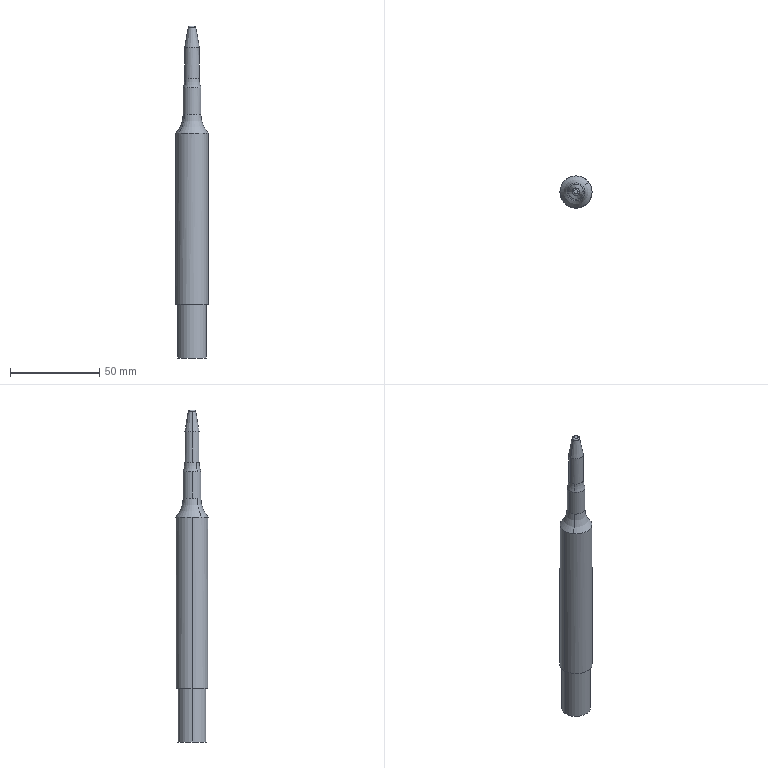Part | 1 solid | 19 faces | box 18 x 18 x 186 mm | volume 34533 mm3 | cylinder 8 | torus 6 | plane 3 | cone 2 | commonest cylinder face diameters 8.2 x2 9.9 x2 16 x2 18 x2
STEP:
#1=CARTESIAN_POINT('',(0.,0.,0.));
#2=DIRECTION('',(0.,0.,1.));
#3=DIRECTION('',(1.,0.,0.));
#4=AXIS2_PLACEMENT_3D('',#1,#2,#3);
#5=CARTESIAN_POINT('',(-232.,180.5,-322.55));
#6=VERTEX_POINT('',#5);
#7=CARTESIAN_POINT('',(-248.,180.5,-322.55));
#8=VERTEX_POINT('',#7);
#9=CARTESIAN_POINT('',(-240.,180.5,-322.55));
#10=DIRECTION('',(0.,0.,1.));
#11=DIRECTION('',(1.,0.,0.));
#12=AXIS2_PLACEMENT_3D('',#9,#10,#11);
#13=CIRCLE('',#12,8.);
#14=CARTESIAN_POINT('',(-226.,4.5,-322.55));
#15=DIRECTION('',(0.,0.,1.));
#16=DIRECTION('',(0.,1.,0.));
#17=AXIS2_PLACEMENT_3D('',#14,#15,#16);
#18=PLANE('',#17);
#19=CARTESIAN_POINT('',(176.,14.));
#20=DIRECTION('',(0.,-1.));
#21=AXIS2_PLACEMENT_2D('',#19,#20);
#22=CIRCLE('',#21,8.);
#23=(GEOMETRIC_REPRESENTATION_CONTEXT(2)PARAMETRIC_REPRESENTATION_CONTEXT()REPRESENTATION_CONTEXT('',''));
#24=DEFINITIONAL_REPRESENTATION('',(#22),#23);
#25=PCURVE('',#18,#24);
#26=CARTESIAN_POINT('',(-240.,180.5,-342.55));
#27=DIRECTION('',(0.,0.,1.));
#28=DIRECTION('',(0.,-1.,0.));
#29=AXIS2_PLACEMENT_3D('',#26,#27,#28);
#30=CYLINDRICAL_SURFACE('',#29,8.);
#31=CARTESIAN_POINT('',(1.571,20.));
#32=DIRECTION('',(1.,0.));
#33=VECTOR('',#32,1.);
#34=LINE('',#31,#33);
#35=(GEOMETRIC_REPRESENTATION_CONTEXT(2)PARAMETRIC_REPRESENTATION_CONTEXT()REPRESENTATION_CONTEXT('',''));
#36=DEFINITIONAL_REPRESENTATION('',(#34),#35);
#37=PCURVE('',#30,#36);
#38=SURFACE_CURVE('',#13,(#25,#37),.PCURVE_S1.);
#39=EDGE_CURVE('',#6,#8,#38,.T.);
#40=ORIENTED_EDGE('',*,*,#39,.T.);
#41=CARTESIAN_POINT('',(-240.,180.5,-322.55));
#42=DIRECTION('',(0.,0.,1.));
#43=DIRECTION('',(1.,0.,0.));
#44=AXIS2_PLACEMENT_3D('',#41,#42,#43);
#45=CIRCLE('',#44,8.);
#46=CARTESIAN_POINT('',(176.,14.));
#47=DIRECTION('',(0.,-1.));
#48=AXIS2_PLACEMENT_2D('',#46,#47);
#49=CIRCLE('',#48,8.);
#50=(GEOMETRIC_REPRESENTATION_CONTEXT(2)PARAMETRIC_REPRESENTATION_CONTEXT()REPRESENTATION_CONTEXT('',''));
#51=DEFINITIONAL_REPRESENTATION('',(#49),#50);
#52=PCURVE('',#18,#51);
#53=CARTESIAN_POINT('',(-240.,180.5,-342.55));
#54=DIRECTION('',(0.,0.,1.));
#55=DIRECTION('',(0.,1.,0.));
#56=AXIS2_PLACEMENT_3D('',#53,#54,#55);
#57=CYLINDRICAL_SURFACE('',#56,8.);
#58=CARTESIAN_POINT('',(-1.571,20.));
#59=DIRECTION('',(1.,0.));
#60=VECTOR('',#59,1.);
#61=LINE('',#58,#60);
#62=(GEOMETRIC_REPRESENTATION_CONTEXT(2)PARAMETRIC_REPRESENTATION_CONTEXT()REPRESENTATION_CONTEXT('',''));
#63=DEFINITIONAL_REPRESENTATION('',(#61),#62);
#64=PCURVE('',#57,#63);
#65=SURFACE_CURVE('',#45,(#52,#64),.PCURVE_S1.);
#66=EDGE_CURVE('',#8,#6,#65,.T.);
#67=ORIENTED_EDGE('',*,*,#66,.T.);
#68=EDGE_LOOP('',(#40,#67));
#69=FACE_BOUND('',#68,.T.);
#70=CARTESIAN_POINT('',(-231.,180.5,-322.55));
#71=VERTEX_POINT('',#70);
#72=CARTESIAN_POINT('',(-249.,180.5,-322.55));
#73=VERTEX_POINT('',#72);
#74=CARTESIAN_POINT('',(-240.,180.5,-322.55));
#75=DIRECTION('',(0.,0.,1.));
#76=DIRECTION('',(-1.,0.,0.));
#77=AXIS2_PLACEMENT_3D('',#74,#75,#76);
#78=CIRCLE('',#77,9.);
#79=CARTESIAN_POINT('',(176.,14.));
#80=DIRECTION('',(0.,1.));
#81=AXIS2_PLACEMENT_2D('',#79,#80);
#82=CIRCLE('',#81,9.);
#83=(GEOMETRIC_REPRESENTATION_CONTEXT(2)PARAMETRIC_REPRESENTATION_CONTEXT()REPRESENTATION_CONTEXT('',''));
#84=DEFINITIONAL_REPRESENTATION('',(#82),#83);
#85=PCURVE('',#18,#84);
#86=CARTESIAN_POINT('',(-240.,180.5,-306.55));
#87=DIRECTION('',(0.,0.,1.));
#88=DIRECTION('',(0.,-1.,0.));
#89=AXIS2_PLACEMENT_3D('',#86,#87,#88);
#90=CYLINDRICAL_SURFACE('',#89,9.);
#91=CARTESIAN_POINT('',(-1.571,-16.));
#92=DIRECTION('',(1.,0.));
#93=VECTOR('',#92,1.);
#94=LINE('',#91,#93);
#95=(GEOMETRIC_REPRESENTATION_CONTEXT(2)PARAMETRIC_REPRESENTATION_CONTEXT()REPRESENTATION_CONTEXT('',''));
#96=DEFINITIONAL_REPRESENTATION('',(#94),#95);
#97=PCURVE('',#90,#96);
#98=SURFACE_CURVE('',#78,(#85,#97),.PCURVE_S1.);
#99=EDGE_CURVE('',#71,#73,#98,.T.);
#100=ORIENTED_EDGE('',*,*,#99,.F.);
#101=CARTESIAN_POINT('',(-240.,180.5,-322.55));
#102=DIRECTION('',(0.,0.,1.));
#103=DIRECTION('',(-1.,0.,0.));
#104=AXIS2_PLACEMENT_3D('',#101,#102,#103);
#105=CIRCLE('',#104,9.);
#106=CARTESIAN_POINT('',(176.,14.));
#107=DIRECTION('',(0.,1.));
#108=AXIS2_PLACEMENT_2D('',#106,#107);
#109=CIRCLE('',#108,9.);
#110=(GEOMETRIC_REPRESENTATION_CONTEXT(2)PARAMETRIC_REPRESENTATION_CONTEXT()REPRESENTATION_CONTEXT('',''));
#111=DEFINITIONAL_REPRESENTATION('',(#109),#110);
#112=PCURVE('',#18,#111);
#113=CARTESIAN_POINT('',(-240.,180.5,-306.55));
#114=DIRECTION('',(0.,0.,1.));
#115=DIRECTION('',(0.,1.,0.));
#116=AXIS2_PLACEMENT_3D('',#113,#114,#115);
#117=CYLINDRICAL_SURFACE('',#116,9.);
#118=CARTESIAN_POINT('',(1.571,-16.));
#119=DIRECTION('',(1.,0.));
#120=VECTOR('',#119,1.);
#121=LINE('',#118,#120);
#122=(GEOMETRIC_REPRESENTATION_CONTEXT(2)PARAMETRIC_REPRESENTATION_CONTEXT()REPRESENTATION_CONTEXT('',''));
#123=DEFINITIONAL_REPRESENTATION('',(#121),#122);
#124=PCURVE('',#117,#123);
#125=SURFACE_CURVE('',#105,(#112,#124),.PCURVE_S1.);
#126=EDGE_CURVE('',#73,#71,#125,.T.);
#127=ORIENTED_EDGE('',*,*,#126,.F.);
#128=EDGE_LOOP('',(#100,#127));
#129=FACE_BOUND('',#128,.T.);
#130=ADVANCED_FACE('',(#69,#129),#18,.F.);
#131=CARTESIAN_POINT('',(-231.,180.5,-226.55));
#132=VERTEX_POINT('',#131);
#133=CARTESIAN_POINT('',(-231.,180.5,-322.55));
#134=DIRECTION('',(0.,0.,1.));
#135=VECTOR('',#134,1.);
#136=LINE('',#133,#135);
#137=CARTESIAN_POINT('',(1.571,-16.));
#138=DIRECTION('',(0.,1.));
#139=VECTOR('',#138,1.);
#140=LINE('',#137,#139);
#141=(GEOMETRIC_REPRESENTATION_CONTEXT(2)PARAMETRIC_REPRESENTATION_CONTEXT()REPRESENTATION_CONTEXT('',''));
#142=DEFINITIONAL_REPRESENTATION('',(#140),#141);
#143=PCURVE('',#90,#142);
#144=CARTESIAN_POINT('',(4.712,-16.));
#145=DIRECTION('',(0.,1.));
#146=VECTOR('',#145,1.);
#147=LINE('',#144,#146);
#148=(GEOMETRIC_REPRESENTATION_CONTEXT(2)PARAMETRIC_REPRESENTATION_CONTEXT()REPRESENTATION_CONTEXT('',''));
#149=DEFINITIONAL_REPRESENTATION('',(#147),#148);
#150=PCURVE('',#117,#149);
#151=SURFACE_CURVE('',#136,(#143,#150),.PCURVE_S1.);
#152=EDGE_CURVE('',#71,#132,#151,.T.);
#153=ORIENTED_EDGE('',*,*,#152,.F.);
#154=ORIENTED_EDGE('',*,*,#99,.T.);
#155=CARTESIAN_POINT('',(-249.,180.5,-226.55));
#156=VERTEX_POINT('',#155);
#157=CARTESIAN_POINT('',(-249.,180.5,-322.55));
#158=DIRECTION('',(0.,0.,1.));
#159=VECTOR('',#158,1.);
#160=LINE('',#157,#159);
#161=CARTESIAN_POINT('',(4.712,-16.));
#162=DIRECTION('',(0.,1.));
#163=VECTOR('',#162,1.);
#164=LINE('',#161,#163);
#165=(GEOMETRIC_REPRESENTATION_CONTEXT(2)PARAMETRIC_REPRESENTATION_CONTEXT()REPRESENTATION_CONTEXT('',''));
#166=DEFINITIONAL_REPRESENTATION('',(#164),#165);
#167=PCURVE('',#90,#166);
#168=CARTESIAN_POINT('',(1.571,-16.));
#169=DIRECTION('',(0.,1.));
#170=VECTOR('',#169,1.);
#171=LINE('',#168,#170);
#172=(GEOMETRIC_REPRESENTATION_CONTEXT(2)PARAMETRIC_REPRESENTATION_CONTEXT()REPRESENTATION_CONTEXT('',''));
#173=DEFINITIONAL_REPRESENTATION('',(#171),#172);
#174=PCURVE('',#117,#173);
#175=SURFACE_CURVE('',#160,(#167,#174),.PCURVE_S1.);
#176=EDGE_CURVE('',#73,#156,#175,.T.);
#177=ORIENTED_EDGE('',*,*,#176,.T.);
#178=CARTESIAN_POINT('',(-232.719,185.79,-226.55));
#179=VERTEX_POINT('',#178);
#180=CARTESIAN_POINT('',(-240.,180.5,-226.55));
#181=DIRECTION('',(0.,0.,-1.));
#182=DIRECTION('',(-1.,0.,0.));
#183=AXIS2_PLACEMENT_3D('',#180,#181,#182);
#184=CIRCLE('',#183,9.);
#185=CARTESIAN_POINT('',(4.712,80.));
#186=DIRECTION('',(-1.,0.));
#187=VECTOR('',#186,1.);
#188=LINE('',#185,#187);
#189=(GEOMETRIC_REPRESENTATION_CONTEXT(2)PARAMETRIC_REPRESENTATION_CONTEXT()REPRESENTATION_CONTEXT('',''));
#190=DEFINITIONAL_REPRESENTATION('',(#188),#189);
#191=PCURVE('',#90,#190);
#192=CARTESIAN_POINT('',(-240.,180.5,-215.911));
#193=DIRECTION('',(0.,0.,-1.));
#194=DIRECTION('',(0.5878,-0.809,0.));
#195=AXIS2_PLACEMENT_3D('',#192,#193,#194);
#196=TOROIDAL_SURFACE('',#195,20.95,16.);
#197=CARTESIAN_POINT('',(2.199,2.414));
#198=DIRECTION('',(1.,0.));
#199=VECTOR('',#198,1.);
#200=LINE('',#197,#199);
#201=(GEOMETRIC_REPRESENTATION_CONTEXT(2)PARAMETRIC_REPRESENTATION_CONTEXT()REPRESENTATION_CONTEXT('',''));
#202=DEFINITIONAL_REPRESENTATION('',(#200),#201);
#203=PCURVE('',#196,#202);
#204=SURFACE_CURVE('',#184,(#191,#203),.PCURVE_S1.);
#205=EDGE_CURVE('',#156,#179,#204,.T.);
#206=ORIENTED_EDGE('',*,*,#205,.T.);
#207=CARTESIAN_POINT('',(-240.,180.5,-226.55));
#208=DIRECTION('',(0.,0.,-1.));
#209=DIRECTION('',(-1.,0.,0.));
#210=AXIS2_PLACEMENT_3D('',#207,#208,#209);
#211=CIRCLE('',#210,9.);
#212=CARTESIAN_POINT('',(4.712,80.));
#213=DIRECTION('',(-1.,0.));
#214=VECTOR('',#213,1.);
#215=LINE('',#212,#214);
#216=(GEOMETRIC_REPRESENTATION_CONTEXT(2)PARAMETRIC_REPRESENTATION_CONTEXT()REPRESENTATION_CONTEXT('',''));
#217=DEFINITIONAL_REPRESENTATION('',(#215),#216);
#218=PCURVE('',#90,#217);
#219=CARTESIAN_POINT('',(-240.,180.5,-215.911));
#220=DIRECTION('',(0.,0.,-1.));
#221=DIRECTION('',(-0.5878,0.809,0.));
#222=AXIS2_PLACEMENT_3D('',#219,#220,#221);
#223=TOROIDAL_SURFACE('',#222,20.95,16.);
#224=CARTESIAN_POINT('',(-0.9425,2.414));
#225=DIRECTION('',(1.,0.));
#226=VECTOR('',#225,1.);
#227=LINE('',#224,#226);
#228=(GEOMETRIC_REPRESENTATION_CONTEXT(2)PARAMETRIC_REPRESENTATION_CONTEXT()REPRESENTATION_CONTEXT('',''));
#229=DEFINITIONAL_REPRESENTATION('',(#227),#228);
#230=PCURVE('',#223,#229);
#231=SURFACE_CURVE('',#211,(#218,#230),.PCURVE_S1.);
#232=EDGE_CURVE('',#179,#132,#231,.T.);
#233=ORIENTED_EDGE('',*,*,#232,.T.);
#234=EDGE_LOOP('',(#153,#154,#177,#206,#233));
#235=FACE_BOUND('',#234,.T.);
#236=ADVANCED_FACE('',(#235),#90,.T.);
#237=ORIENTED_EDGE('',*,*,#232,.T.);
#238=CARTESIAN_POINT('',(-247.281,175.21,-226.55));
#239=VERTEX_POINT('',#238);
#240=CARTESIAN_POINT('',(-240.,180.5,-226.55));
#241=DIRECTION('',(0.,0.,-1.));
#242=DIRECTION('',(-1.,0.,0.));
#243=AXIS2_PLACEMENT_3D('',#240,#241,#242);
#244=CIRCLE('',#243,9.);
#245=CARTESIAN_POINT('',(-0.9425,2.414));
#246=DIRECTION('',(1.,0.));
#247=VECTOR('',#246,1.);
#248=LINE('',#245,#247);
#249=(GEOMETRIC_REPRESENTATION_CONTEXT(2)PARAMETRIC_REPRESENTATION_CONTEXT()REPRESENTATION_CONTEXT('',''));
#250=DEFINITIONAL_REPRESENTATION('',(#248),#249);
#251=PCURVE('',#223,#250);
#252=CARTESIAN_POINT('',(7.854,80.));
#253=DIRECTION('',(-1.,0.));
#254=VECTOR('',#253,1.);
#255=LINE('',#252,#254);
#256=(GEOMETRIC_REPRESENTATION_CONTEXT(2)PARAMETRIC_REPRESENTATION_CONTEXT()REPRESENTATION_CONTEXT('',''));
#257=DEFINITIONAL_REPRESENTATION('',(#255),#256);
#258=PCURVE('',#117,#257);
#259=SURFACE_CURVE('',#244,(#251,#258),.PCURVE_S1.);
#260=EDGE_CURVE('',#132,#239,#259,.T.);
#261=ORIENTED_EDGE('',*,*,#260,.T.);
#262=CARTESIAN_POINT('',(-244.005,177.591,-215.911));
#263=VERTEX_POINT('',#262);
#264=CARTESIAN_POINT('',(-256.949,168.186,-215.911));
#265=DIRECTION('',(-0.5878,0.809,0.));
#266=DIRECTION('',(0.809,0.5878,0.));
#267=AXIS2_PLACEMENT_3D('',#264,#265,#266);
#268=CIRCLE('',#267,16.);
#269=CARTESIAN_POINT('',(4.712,3.142));
#270=DIRECTION('',(0.,-1.));
#271=VECTOR('',#270,1.);
#272=LINE('',#269,#271);
#273=(GEOMETRIC_REPRESENTATION_CONTEXT(2)PARAMETRIC_REPRESENTATION_CONTEXT()REPRESENTATION_CONTEXT('',''));
#274=DEFINITIONAL_REPRESENTATION('',(#272),#273);
#275=PCURVE('',#223,#274);
#276=CARTESIAN_POINT('',(1.571,3.142));
#277=DIRECTION('',(0.,-1.));
#278=VECTOR('',#277,1.);
#279=LINE('',#276,#278);
#280=(GEOMETRIC_REPRESENTATION_CONTEXT(2)PARAMETRIC_REPRESENTATION_CONTEXT()REPRESENTATION_CONTEXT('',''));
#281=DEFINITIONAL_REPRESENTATION('',(#279),#280);
#282=PCURVE('',#196,#281);
#283=SURFACE_CURVE('',#268,(#275,#282),.PCURVE_S1.);
#284=EDGE_CURVE('',#263,#239,#283,.T.);
#285=ORIENTED_EDGE('',*,*,#284,.F.);
#286=CARTESIAN_POINT('',(-235.995,177.591,-215.911));
#287=VERTEX_POINT('',#286);
#288=CARTESIAN_POINT('',(-240.,180.5,-215.911));
#289=DIRECTION('',(0.,0.,1.));
#290=DIRECTION('',(0.809,-0.5878,0.));
#291=AXIS2_PLACEMENT_3D('',#288,#289,#290);
#292=CIRCLE('',#291,4.95);
#293=CARTESIAN_POINT('',(9.111,3.142));
#294=DIRECTION('',(-1.,0.));
#295=VECTOR('',#294,1.);
#296=LINE('',#293,#295);
#297=(GEOMETRIC_REPRESENTATION_CONTEXT(2)PARAMETRIC_REPRESENTATION_CONTEXT()REPRESENTATION_CONTEXT('',''));
#298=DEFINITIONAL_REPRESENTATION('',(#296),#297);
#299=PCURVE('',#223,#298);
#300=CARTESIAN_POINT('',(-240.,180.5,-306.55));
#301=DIRECTION('',(0.,0.,1.));
#302=DIRECTION('',(0.,1.,0.));
#303=AXIS2_PLACEMENT_3D('',#300,#301,#302);
#304=CYLINDRICAL_SURFACE('',#303,4.95);
#305=CARTESIAN_POINT('',(-2.199,90.639));
#306=DIRECTION('',(1.,0.));
#307=VECTOR('',#306,1.);
#308=LINE('',#305,#307);
#309=(GEOMETRIC_REPRESENTATION_CONTEXT(2)PARAMETRIC_REPRESENTATION_CONTEXT()REPRESENTATION_CONTEXT('',''));
#310=DEFINITIONAL_REPRESENTATION('',(#308),#309);
#311=PCURVE('',#304,#310);
#312=SURFACE_CURVE('',#292,(#299,#311),.PCURVE_S1.);
#313=EDGE_CURVE('',#263,#287,#312,.T.);
#314=ORIENTED_EDGE('',*,*,#313,.T.);
#315=CARTESIAN_POINT('',(-235.05,180.5,-215.911));
#316=VERTEX_POINT('',#315);
#317=CARTESIAN_POINT('',(-240.,180.5,-215.911));
#318=DIRECTION('',(0.,0.,1.));
#319=DIRECTION('',(0.809,-0.5878,0.));
#320=AXIS2_PLACEMENT_3D('',#317,#318,#319);
#321=CIRCLE('',#320,4.95);
#322=CARTESIAN_POINT('',(2.827,3.142));
#323=DIRECTION('',(-1.,0.));
#324=VECTOR('',#323,1.);
#325=LINE('',#322,#324);
#326=(GEOMETRIC_REPRESENTATION_CONTEXT(2)PARAMETRIC_REPRESENTATION_CONTEXT()REPRESENTATION_CONTEXT('',''));
#327=DEFINITIONAL_REPRESENTATION('',(#325),#326);
#328=PCURVE('',#223,#327);
#329=CARTESIAN_POINT('',(4.084,90.639));
#330=DIRECTION('',(1.,0.));
#331=VECTOR('',#330,1.);
#332=LINE('',#329,#331);
#333=(GEOMETRIC_REPRESENTATION_CONTEXT(2)PARAMETRIC_REPRESENTATION_CONTEXT()REPRESENTATION_CONTEXT('',''));
#334=DEFINITIONAL_REPRESENTATION('',(#332),#333);
#335=PCURVE('',#304,#334);
#336=SURFACE_CURVE('',#321,(#328,#335),.PCURVE_S1.);
#337=EDGE_CURVE('',#287,#316,#336,.T.);
#338=ORIENTED_EDGE('',*,*,#337,.T.);
#339=CARTESIAN_POINT('',(-235.995,183.41,-215.911));
#340=VERTEX_POINT('',#339);
#341=CARTESIAN_POINT('',(-240.,180.5,-215.911));
#342=DIRECTION('',(0.,0.,1.));
#343=DIRECTION('',(0.809,-0.5878,0.));
#344=AXIS2_PLACEMENT_3D('',#341,#342,#343);
#345=CIRCLE('',#344,4.95);
#346=CARTESIAN_POINT('',(2.827,3.142));
#347=DIRECTION('',(-1.,0.));
#348=VECTOR('',#347,1.);
#349=LINE('',#346,#348);
#350=(GEOMETRIC_REPRESENTATION_CONTEXT(2)PARAMETRIC_REPRESENTATION_CONTEXT()REPRESENTATION_CONTEXT('',''));
#351=DEFINITIONAL_REPRESENTATION('',(#349),#350);
#352=PCURVE('',#223,#351);
#353=CARTESIAN_POINT('',(-240.,180.5,-306.55));
#354=DIRECTION('',(0.,0.,1.));
#355=DIRECTION('',(0.,-1.,0.));
#356=AXIS2_PLACEMENT_3D('',#353,#354,#355);
#357=CYLINDRICAL_SURFACE('',#356,4.95);
#358=CARTESIAN_POINT('',(0.9425,90.639));
#359=DIRECTION('',(1.,0.));
#360=VECTOR('',#359,1.);
#361=LINE('',#358,#360);
#362=(GEOMETRIC_REPRESENTATION_CONTEXT(2)PARAMETRIC_REPRESENTATION_CONTEXT()REPRESENTATION_CONTEXT('',''));
#363=DEFINITIONAL_REPRESENTATION('',(#361),#362);
#364=PCURVE('',#357,#363);
#365=SURFACE_CURVE('',#345,(#352,#364),.PCURVE_S1.);
#366=EDGE_CURVE('',#316,#340,#365,.T.);
#367=ORIENTED_EDGE('',*,*,#366,.T.);
#368=CARTESIAN_POINT('',(-223.051,192.814,-215.911));
#369=DIRECTION('',(0.5878,-0.809,0.));
#370=DIRECTION('',(-0.809,-0.5878,0.));
#371=AXIS2_PLACEMENT_3D('',#368,#369,#370);
#372=CIRCLE('',#371,16.);
#373=CARTESIAN_POINT('',(1.571,3.142));
#374=DIRECTION('',(0.,-1.));
#375=VECTOR('',#374,1.);
#376=LINE('',#373,#375);
#377=(GEOMETRIC_REPRESENTATION_CONTEXT(2)PARAMETRIC_REPRESENTATION_CONTEXT()REPRESENTATION_CONTEXT('',''));
#378=DEFINITIONAL_REPRESENTATION('',(#376),#377);
#379=PCURVE('',#223,#378);
#380=CARTESIAN_POINT('',(4.712,3.142));
#381=DIRECTION('',(0.,-1.));
#382=VECTOR('',#381,1.);
#383=LINE('',#380,#382);
#384=(GEOMETRIC_REPRESENTATION_CONTEXT(2)PARAMETRIC_REPRESENTATION_CONTEXT()REPRESENTATION_CONTEXT('',''));
#385=DEFINITIONAL_REPRESENTATION('',(#383),#384);
#386=PCURVE('',#196,#385);
#387=SURFACE_CURVE('',#372,(#379,#386),.PCURVE_S1.);
#388=EDGE_CURVE('',#340,#179,#387,.T.);
#389=ORIENTED_EDGE('',*,*,#388,.T.);
#390=EDGE_LOOP('',(#237,#261,#285,#314,#338,#367,#389));
#391=FACE_BOUND('',#390,.F.);
#392=ADVANCED_FACE('',(#391),#223,.F.);
#393=CARTESIAN_POINT('',(-235.05,180.5,-201.05));
#394=VERTEX_POINT('',#393);
#395=CARTESIAN_POINT('',(-235.05,180.5,-215.911));
#396=DIRECTION('',(0.,0.,1.));
#397=VECTOR('',#396,1.);
#398=LINE('',#395,#397);
#399=CARTESIAN_POINT('',(1.571,90.639));
#400=DIRECTION('',(0.,1.));
#401=VECTOR('',#400,1.);
#402=LINE('',#399,#401);
#403=(GEOMETRIC_REPRESENTATION_CONTEXT(2)PARAMETRIC_REPRESENTATION_CONTEXT()REPRESENTATION_CONTEXT('',''));
#404=DEFINITIONAL_REPRESENTATION('',(#402),#403);
#405=PCURVE('',#357,#404);
#406=CARTESIAN_POINT('',(4.712,90.639));
#407=DIRECTION('',(0.,1.));
#408=VECTOR('',#407,1.);
#409=LINE('',#406,#408);
#410=(GEOMETRIC_REPRESENTATION_CONTEXT(2)PARAMETRIC_REPRESENTATION_CONTEXT()REPRESENTATION_CONTEXT('',''));
#411=DEFINITIONAL_REPRESENTATION('',(#409),#410);
#412=PCURVE('',#304,#411);
#413=SURFACE_CURVE('',#398,(#405,#412),.PCURVE_S1.);
#414=EDGE_CURVE('',#316,#394,#413,.T.);
#415=ORIENTED_EDGE('',*,*,#414,.F.);
#416=ORIENTED_EDGE('',*,*,#366,.T.);
#417=CARTESIAN_POINT('',(-244.95,180.5,-215.911));
#418=VERTEX_POINT('',#417);
#419=CARTESIAN_POINT('',(-240.,180.5,-215.911));
#420=DIRECTION('',(0.,0.,1.));
#421=DIRECTION('',(0.809,-0.5878,0.));
#422=AXIS2_PLACEMENT_3D('',#419,#420,#421);
#423=CIRCLE('',#422,4.95);
#424=CARTESIAN_POINT('',(0.9425,90.639));
#425=DIRECTION('',(1.,0.));
#426=VECTOR('',#425,1.);
#427=LINE('',#424,#426);
#428=(GEOMETRIC_REPRESENTATION_CONTEXT(2)PARAMETRIC_REPRESENTATION_CONTEXT()REPRESENTATION_CONTEXT('',''));
#429=DEFINITIONAL_REPRESENTATION('',(#427),#428);
#430=PCURVE('',#357,#429);
#431=CARTESIAN_POINT('',(5.969,3.142));
#432=DIRECTION('',(-1.,0.));
#433=VECTOR('',#432,1.);
#434=LINE('',#431,#433);
#435=(GEOMETRIC_REPRESENTATION_CONTEXT(2)PARAMETRIC_REPRESENTATION_CONTEXT()REPRESENTATION_CONTEXT('',''));
#436=DEFINITIONAL_REPRESENTATION('',(#434),#435);
#437=PCURVE('',#196,#436);
#438=SURFACE_CURVE('',#423,(#430,#437),.PCURVE_S1.);
#439=EDGE_CURVE('',#340,#418,#438,.T.);
#440=ORIENTED_EDGE('',*,*,#439,.T.);
#441=CARTESIAN_POINT('',(-244.95,180.5,-201.05));
#442=VERTEX_POINT('',#441);
#443=CARTESIAN_POINT('',(-244.95,180.5,-215.911));
#444=DIRECTION('',(0.,0.,1.));
#445=VECTOR('',#444,1.);
#446=LINE('',#443,#445);
#447=CARTESIAN_POINT('',(4.712,90.639));
#448=DIRECTION('',(0.,1.));
#449=VECTOR('',#448,1.);
#450=LINE('',#447,#449);
#451=(GEOMETRIC_REPRESENTATION_CONTEXT(2)PARAMETRIC_REPRESENTATION_CONTEXT()REPRESENTATION_CONTEXT('',''));
#452=DEFINITIONAL_REPRESENTATION('',(#450),#451);
#453=PCURVE('',#357,#452);
#454=CARTESIAN_POINT('',(1.571,90.639));
#455=DIRECTION('',(0.,1.));
#456=VECTOR('',#455,1.);
#457=LINE('',#454,#456);
#458=(GEOMETRIC_REPRESENTATION_CONTEXT(2)PARAMETRIC_REPRESENTATION_CONTEXT()REPRESENTATION_CONTEXT('',''));
#459=DEFINITIONAL_REPRESENTATION('',(#457),#458);
#460=PCURVE('',#304,#459);
#461=SURFACE_CURVE('',#446,(#453,#460),.PCURVE_S1.);
#462=EDGE_CURVE('',#418,#442,#461,.T.);
#463=ORIENTED_EDGE('',*,*,#462,.T.);
#464=CARTESIAN_POINT('',(-235.995,183.41,-201.05));
#465=VERTEX_POINT('',#464);
#466=CARTESIAN_POINT('',(-240.,180.5,-201.05));
#467=DIRECTION('',(0.,0.,1.));
#468=DIRECTION('',(1.,0.,0.));
#469=AXIS2_PLACEMENT_3D('',#466,#467,#468);
#470=CIRCLE('',#469,4.95);
#471=CARTESIAN_POINT('',(1.571,105.5));
#472=DIRECTION('',(1.,0.));
#473=VECTOR('',#472,1.);
#474=LINE('',#471,#473);
#475=(GEOMETRIC_REPRESENTATION_CONTEXT(2)PARAMETRIC_REPRESENTATION_CONTEXT()REPRESENTATION_CONTEXT('',''));
#476=DEFINITIONAL_REPRESENTATION('',(#474),#475);
#477=PCURVE('',#357,#476);
#478=CARTESIAN_POINT('',(-240.,180.5,-195.904));
#479=DIRECTION('',(0.,0.,-1.));
#480=DIRECTION('',(0.5878,-0.809,0.));
#481=AXIS2_PLACEMENT_3D('',#478,#479,#480);
#482=TOROIDAL_SURFACE('',#481,20.1,16.);
#483=CARTESIAN_POINT('',(5.341,2.814));
#484=DIRECTION('',(-1.,0.));
#485=VECTOR('',#484,1.);
#486=LINE('',#483,#485);
#487=(GEOMETRIC_REPRESENTATION_CONTEXT(2)PARAMETRIC_REPRESENTATION_CONTEXT()REPRESENTATION_CONTEXT('',''));
#488=DEFINITIONAL_REPRESENTATION('',(#486),#487);
#489=PCURVE('',#482,#488);
#490=SURFACE_CURVE('',#470,(#477,#489),.PCURVE_S1.);
#491=EDGE_CURVE('',#465,#442,#490,.T.);
#492=ORIENTED_EDGE('',*,*,#491,.F.);
#493=CARTESIAN_POINT('',(-240.,180.5,-201.05));
#494=DIRECTION('',(0.,0.,1.));
#495=DIRECTION('',(1.,0.,0.));
#496=AXIS2_PLACEMENT_3D('',#493,#494,#495);
#497=CIRCLE('',#496,4.95);
#498=CARTESIAN_POINT('',(1.571,105.5));
#499=DIRECTION('',(1.,0.));
#500=VECTOR('',#499,1.);
#501=LINE('',#498,#500);
#502=(GEOMETRIC_REPRESENTATION_CONTEXT(2)PARAMETRIC_REPRESENTATION_CONTEXT()REPRESENTATION_CONTEXT('',''));
#503=DEFINITIONAL_REPRESENTATION('',(#501),#502);
#504=PCURVE('',#357,#503);
#505=CARTESIAN_POINT('',(-240.,180.5,-195.904));
#506=DIRECTION('',(0.,0.,-1.));
#507=DIRECTION('',(-0.5878,0.809,0.));
#508=AXIS2_PLACEMENT_3D('',#505,#506,#507);
#509=TOROIDAL_SURFACE('',#508,20.1,16.);
#510=CARTESIAN_POINT('',(2.199,2.814));
#511=DIRECTION('',(-1.,0.));
#512=VECTOR('',#511,1.);
#513=LINE('',#510,#512);
#514=(GEOMETRIC_REPRESENTATION_CONTEXT(2)PARAMETRIC_REPRESENTATION_CONTEXT()REPRESENTATION_CONTEXT('',''));
#515=DEFINITIONAL_REPRESENTATION('',(#513),#514);
#516=PCURVE('',#509,#515);
#517=SURFACE_CURVE('',#497,(#504,#516),.PCURVE_S1.);
#518=EDGE_CURVE('',#394,#465,#517,.T.);
#519=ORIENTED_EDGE('',*,*,#518,.F.);
#520=EDGE_LOOP('',(#415,#416,#440,#463,#492,#519));
#521=FACE_BOUND('',#520,.T.);
#522=ADVANCED_FACE('',(#521),#357,.T.);
#523=ORIENTED_EDGE('',*,*,#518,.F.);
#524=CARTESIAN_POINT('',(-244.005,177.591,-201.05));
#525=VERTEX_POINT('',#524);
#526=CARTESIAN_POINT('',(-240.,180.5,-201.05));
#527=DIRECTION('',(0.,0.,1.));
#528=DIRECTION('',(1.,0.,0.));
#529=AXIS2_PLACEMENT_3D('',#526,#527,#528);
#530=CIRCLE('',#529,4.95);
#531=CARTESIAN_POINT('',(8.482,2.814));
#532=DIRECTION('',(-1.,0.));
#533=VECTOR('',#532,1.);
#534=LINE('',#531,#533);
#535=(GEOMETRIC_REPRESENTATION_CONTEXT(2)PARAMETRIC_REPRESENTATION_CONTEXT()REPRESENTATION_CONTEXT('',''));
#536=DEFINITIONAL_REPRESENTATION('',(#534),#535);
#537=PCURVE('',#509,#536);
#538=CARTESIAN_POINT('',(-1.571,105.5));
#539=DIRECTION('',(1.,0.));
#540=VECTOR('',#539,1.);
#541=LINE('',#538,#540);
#542=(GEOMETRIC_REPRESENTATION_CONTEXT(2)PARAMETRIC_REPRESENTATION_CONTEXT()REPRESENTATION_CONTEXT('',''));
#543=DEFINITIONAL_REPRESENTATION('',(#541),#542);
#544=PCURVE('',#304,#543);
#545=SURFACE_CURVE('',#530,(#537,#544),.PCURVE_S1.);
#546=EDGE_CURVE('',#525,#394,#545,.T.);
#547=ORIENTED_EDGE('',*,*,#546,.F.);
#548=CARTESIAN_POINT('',(-243.317,178.09,-195.904));
#549=VERTEX_POINT('',#548);
#550=CARTESIAN_POINT('',(-256.261,168.686,-195.904));
#551=DIRECTION('',(-0.5878,0.809,0.));
#552=DIRECTION('',(0.809,0.5878,0.));
#553=AXIS2_PLACEMENT_3D('',#550,#551,#552);
#554=CIRCLE('',#553,16.);
#555=CARTESIAN_POINT('',(4.712,3.142));
#556=DIRECTION('',(0.,-1.));
#557=VECTOR('',#556,1.);
#558=LINE('',#555,#557);
#559=(GEOMETRIC_REPRESENTATION_CONTEXT(2)PARAMETRIC_REPRESENTATION_CONTEXT()REPRESENTATION_CONTEXT('',''));
#560=DEFINITIONAL_REPRESENTATION('',(#558),#559);
#561=PCURVE('',#509,#560);
#562=CARTESIAN_POINT('',(1.571,3.142));
#563=DIRECTION('',(0.,-1.));
#564=VECTOR('',#563,1.);
#565=LINE('',#562,#564);
#566=(GEOMETRIC_REPRESENTATION_CONTEXT(2)PARAMETRIC_REPRESENTATION_CONTEXT()REPRESENTATION_CONTEXT('',''));
#567=DEFINITIONAL_REPRESENTATION('',(#565),#566);
#568=PCURVE('',#482,#567);
#569=SURFACE_CURVE('',#554,(#561,#568),.PCURVE_S1.);
#570=EDGE_CURVE('',#549,#525,#569,.T.);
#571=ORIENTED_EDGE('',*,*,#570,.F.);
#572=CARTESIAN_POINT('',(-235.9,180.5,-195.904));
#573=VERTEX_POINT('',#572);
#574=CARTESIAN_POINT('',(-240.,180.5,-195.904));
#575=DIRECTION('',(0.,0.,1.));
#576=DIRECTION('',(-1.,0.,0.));
#577=AXIS2_PLACEMENT_3D('',#574,#575,#576);
#578=CIRCLE('',#577,4.1);
#579=CARTESIAN_POINT('',(5.341,3.142));
#580=DIRECTION('',(-1.,0.));
#581=VECTOR('',#580,1.);
#582=LINE('',#579,#581);
#583=(GEOMETRIC_REPRESENTATION_CONTEXT(2)PARAMETRIC_REPRESENTATION_CONTEXT()REPRESENTATION_CONTEXT('',''));
#584=DEFINITIONAL_REPRESENTATION('',(#582),#583);
#585=PCURVE('',#509,#584);
#586=CARTESIAN_POINT('',(-240.,180.5,-169.55));
#587=DIRECTION('',(0.,0.,-1.));
#588=DIRECTION('',(0.,1.,0.));
#589=AXIS2_PLACEMENT_3D('',#586,#587,#588);
#590=CYLINDRICAL_SURFACE('',#589,4.1);
#591=CARTESIAN_POINT('',(4.712,26.354));
#592=DIRECTION('',(-1.,0.));
#593=VECTOR('',#592,1.);
#594=LINE('',#591,#593);
#595=(GEOMETRIC_REPRESENTATION_CONTEXT(2)PARAMETRIC_REPRESENTATION_CONTEXT()REPRESENTATION_CONTEXT('',''));
#596=DEFINITIONAL_REPRESENTATION('',(#594),#595);
#597=PCURVE('',#590,#596);
#598=SURFACE_CURVE('',#578,(#585,#597),.PCURVE_S1.);
#599=EDGE_CURVE('',#549,#573,#598,.T.);
#600=ORIENTED_EDGE('',*,*,#599,.T.);
#601=CARTESIAN_POINT('',(-236.683,182.91,-195.904));
#602=VERTEX_POINT('',#601);
#603=CARTESIAN_POINT('',(-240.,180.5,-195.904));
#604=DIRECTION('',(0.,0.,1.));
#605=DIRECTION('',(-1.,0.,0.));
#606=AXIS2_PLACEMENT_3D('',#603,#604,#605);
#607=CIRCLE('',#606,4.1);
#608=CARTESIAN_POINT('',(5.341,3.142));
#609=DIRECTION('',(-1.,0.));
#610=VECTOR('',#609,1.);
#611=LINE('',#608,#610);
#612=(GEOMETRIC_REPRESENTATION_CONTEXT(2)PARAMETRIC_REPRESENTATION_CONTEXT()REPRESENTATION_CONTEXT('',''));
#613=DEFINITIONAL_REPRESENTATION('',(#611),#612);
#614=PCURVE('',#509,#613);
#615=CARTESIAN_POINT('',(-240.,180.5,-169.55));
#616=DIRECTION('',(0.,0.,-1.));
#617=DIRECTION('',(0.,-1.,0.));
#618=AXIS2_PLACEMENT_3D('',#615,#616,#617);
#619=CYLINDRICAL_SURFACE('',#618,4.1);
#620=CARTESIAN_POINT('',(7.854,26.354));
#621=DIRECTION('',(-1.,0.));
#622=VECTOR('',#621,1.);
#623=LINE('',#620,#622);
#624=(GEOMETRIC_REPRESENTATION_CONTEXT(2)PARAMETRIC_REPRESENTATION_CONTEXT()REPRESENTATION_CONTEXT('',''));
#625=DEFINITIONAL_REPRESENTATION('',(#623),#624);
#626=PCURVE('',#619,#625);
#627=SURFACE_CURVE('',#607,(#614,#626),.PCURVE_S1.);
#628=EDGE_CURVE('',#573,#602,#627,.T.);
#629=ORIENTED_EDGE('',*,*,#628,.T.);
#630=CARTESIAN_POINT('',(-223.739,192.315,-195.904));
#631=DIRECTION('',(0.5878,-0.809,0.));
#632=DIRECTION('',(-0.809,-0.5878,0.));
#633=AXIS2_PLACEMENT_3D('',#630,#631,#632);
#634=CIRCLE('',#633,16.);
#635=CARTESIAN_POINT('',(1.571,3.142));
#636=DIRECTION('',(0.,-1.));
#637=VECTOR('',#636,1.);
#638=LINE('',#635,#637);
#639=(GEOMETRIC_REPRESENTATION_CONTEXT(2)PARAMETRIC_REPRESENTATION_CONTEXT()REPRESENTATION_CONTEXT('',''));
#640=DEFINITIONAL_REPRESENTATION('',(#638),#639);
#641=PCURVE('',#509,#640);
#642=CARTESIAN_POINT('',(4.712,3.142));
#643=DIRECTION('',(0.,-1.));
#644=VECTOR('',#643,1.);
#645=LINE('',#642,#644);
#646=(GEOMETRIC_REPRESENTATION_CONTEXT(2)PARAMETRIC_REPRESENTATION_CONTEXT()REPRESENTATION_CONTEXT('',''));
#647=DEFINITIONAL_REPRESENTATION('',(#645),#646);
#648=PCURVE('',#482,#647);
#649=SURFACE_CURVE('',#634,(#641,#648),.PCURVE_S1.);
#650=EDGE_CURVE('',#602,#465,#649,.T.);
#651=ORIENTED_EDGE('',*,*,#650,.T.);
#652=EDGE_LOOP('',(#523,#547,#571,#600,#629,#651));
#653=FACE_BOUND('',#652,.F.);
#654=ADVANCED_FACE('',(#653),#509,.F.);
#655=CARTESIAN_POINT('',(-244.1,180.5,-178.6));
#656=VERTEX_POINT('',#655);
#657=CARTESIAN_POINT('',(-244.1,180.5,-195.904));
#658=VERTEX_POINT('',#657);
#659=CARTESIAN_POINT('',(-244.1,180.5,-178.6));
#660=DIRECTION('',(0.,0.,-1.));
#661=VECTOR('',#660,1.);
#662=LINE('',#659,#661);
#663=CARTESIAN_POINT('',(1.571,9.05));
#664=DIRECTION('',(0.,1.));
#665=VECTOR('',#664,1.);
#666=LINE('',#663,#665);
#667=(GEOMETRIC_REPRESENTATION_CONTEXT(2)PARAMETRIC_REPRESENTATION_CONTEXT()REPRESENTATION_CONTEXT('',''));
#668=DEFINITIONAL_REPRESENTATION('',(#666),#667);
#669=PCURVE('',#619,#668);
#670=CARTESIAN_POINT('',(4.712,9.05));
#671=DIRECTION('',(0.,1.));
#672=VECTOR('',#671,1.);
#673=LINE('',#670,#672);
#674=(GEOMETRIC_REPRESENTATION_CONTEXT(2)PARAMETRIC_REPRESENTATION_CONTEXT()REPRESENTATION_CONTEXT('',''));
#675=DEFINITIONAL_REPRESENTATION('',(#673),#674);
#676=PCURVE('',#590,#675);
#677=SURFACE_CURVE('',#662,(#669,#676),.PCURVE_S1.);
#678=EDGE_CURVE('',#656,#658,#677,.T.);
#679=ORIENTED_EDGE('',*,*,#678,.F.);
#680=CARTESIAN_POINT('',(-235.9,180.5,-178.6));
#681=VERTEX_POINT('',#680);
#682=CARTESIAN_POINT('',(-240.,180.5,-178.6));
#683=DIRECTION('',(0.,0.,-1.));
#684=DIRECTION('',(1.,0.,0.));
#685=AXIS2_PLACEMENT_3D('',#682,#683,#684);
#686=CIRCLE('',#685,4.1);
#687=CARTESIAN_POINT('',(-1.571,9.05));
#688=DIRECTION('',(1.,0.));
#689=VECTOR('',#688,1.);
#690=LINE('',#687,#689);
#691=(GEOMETRIC_REPRESENTATION_CONTEXT(2)PARAMETRIC_REPRESENTATION_CONTEXT()REPRESENTATION_CONTEXT('',''));
#692=DEFINITIONAL_REPRESENTATION('',(#690),#691);
#693=PCURVE('',#619,#692);
#694=CARTESIAN_POINT('',(-240.,180.5,-178.6));
#695=DIRECTION('',(0.,0.,-1.));
#696=DIRECTION('',(0.,-1.,0.));
#697=AXIS2_PLACEMENT_3D('',#694,#695,#696);
#698=CONICAL_SURFACE('',#697,4.1,0.1742);
#699=CARTESIAN_POINT('',(-1.571,0.));
#700=DIRECTION('',(1.,0.));
#701=VECTOR('',#700,1.);
#702=LINE('',#699,#701);
#703=(GEOMETRIC_REPRESENTATION_CONTEXT(2)PARAMETRIC_REPRESENTATION_CONTEXT()REPRESENTATION_CONTEXT('',''));
#704=DEFINITIONAL_REPRESENTATION('',(#702),#703);
#705=PCURVE('',#698,#704);
#706=SURFACE_CURVE('',#686,(#693,#705),.PCURVE_S1.);
#707=EDGE_CURVE('',#656,#681,#706,.T.);
#708=ORIENTED_EDGE('',*,*,#707,.T.);
#709=CARTESIAN_POINT('',(-235.9,180.5,-178.6));
#710=DIRECTION('',(0.,0.,-1.));
#711=VECTOR('',#710,1.);
#712=LINE('',#709,#711);
#713=CARTESIAN_POINT('',(4.712,9.05));
#714=DIRECTION('',(0.,1.));
#715=VECTOR('',#714,1.);
#716=LINE('',#713,#715);
#717=(GEOMETRIC_REPRESENTATION_CONTEXT(2)PARAMETRIC_REPRESENTATION_CONTEXT()REPRESENTATION_CONTEXT('',''));
#718=DEFINITIONAL_REPRESENTATION('',(#716),#717);
#719=PCURVE('',#619,#718);
#720=CARTESIAN_POINT('',(1.571,9.05));
#721=DIRECTION('',(0.,1.));
#722=VECTOR('',#721,1.);
#723=LINE('',#720,#722);
#724=(GEOMETRIC_REPRESENTATION_CONTEXT(2)PARAMETRIC_REPRESENTATION_CONTEXT()REPRESENTATION_CONTEXT('',''));
#725=DEFINITIONAL_REPRESENTATION('',(#723),#724);
#726=PCURVE('',#590,#725);
#727=SURFACE_CURVE('',#712,(#719,#726),.PCURVE_S1.);
#728=EDGE_CURVE('',#681,#573,#727,.T.);
#729=ORIENTED_EDGE('',*,*,#728,.T.);
#730=ORIENTED_EDGE('',*,*,#628,.T.);
#731=CARTESIAN_POINT('',(-240.,180.5,-195.904));
#732=DIRECTION('',(0.,0.,1.));
#733=DIRECTION('',(-1.,0.,0.));
#734=AXIS2_PLACEMENT_3D('',#731,#732,#733);
#735=CIRCLE('',#734,4.1);
#736=CARTESIAN_POINT('',(7.854,26.354));
#737=DIRECTION('',(-1.,0.));
#738=VECTOR('',#737,1.);
#739=LINE('',#736,#738);
#740=(GEOMETRIC_REPRESENTATION_CONTEXT(2)PARAMETRIC_REPRESENTATION_CONTEXT()REPRESENTATION_CONTEXT('',''));
#741=DEFINITIONAL_REPRESENTATION('',(#739),#740);
#742=PCURVE('',#619,#741);
#743=CARTESIAN_POINT('',(8.482,3.142));
#744=DIRECTION('',(-1.,0.));
#745=VECTOR('',#744,1.);
#746=LINE('',#743,#745);
#747=(GEOMETRIC_REPRESENTATION_CONTEXT(2)PARAMETRIC_REPRESENTATION_CONTEXT()REPRESENTATION_CONTEXT('',''));
#748=DEFINITIONAL_REPRESENTATION('',(#746),#747);
#749=PCURVE('',#482,#748);
#750=SURFACE_CURVE('',#735,(#742,#749),.PCURVE_S1.);
#751=EDGE_CURVE('',#602,#658,#750,.T.);
#752=ORIENTED_EDGE('',*,*,#751,.T.);
#753=EDGE_LOOP('',(#679,#708,#729,#730,#752));
#754=FACE_BOUND('',#753,.T.);
#755=ADVANCED_FACE('',(#754),#619,.T.);
#756=CARTESIAN_POINT('',(-242.125,180.5,-167.377));
#757=VERTEX_POINT('',#756);
#758=CARTESIAN_POINT('',(-242.125,180.5,-167.377));
#759=DIRECTION('',(-0.1733,0.,-0.9849));
#760=VECTOR('',#759,1.);
#761=LINE('',#758,#760);
#762=CARTESIAN_POINT('',(1.571,-11.223));
#763=DIRECTION('',(0.,1.));
#764=VECTOR('',#763,1.);
#765=LINE('',#762,#764);
#766=(GEOMETRIC_REPRESENTATION_CONTEXT(2)PARAMETRIC_REPRESENTATION_CONTEXT()REPRESENTATION_CONTEXT('',''));
#767=DEFINITIONAL_REPRESENTATION('',(#765),#766);
#768=PCURVE('',#698,#767);
#769=CARTESIAN_POINT('',(-240.,180.5,-178.6));
#770=DIRECTION('',(0.,0.,-1.));
#771=DIRECTION('',(0.,1.,0.));
#772=AXIS2_PLACEMENT_3D('',#769,#770,#771);
#773=CONICAL_SURFACE('',#772,4.1,0.1742);
#774=CARTESIAN_POINT('',(4.712,-11.223));
#775=DIRECTION('',(0.,1.));
#776=VECTOR('',#775,1.);
#777=LINE('',#774,#776);
#778=(GEOMETRIC_REPRESENTATION_CONTEXT(2)PARAMETRIC_REPRESENTATION_CONTEXT()REPRESENTATION_CONTEXT('',''));
#779=DEFINITIONAL_REPRESENTATION('',(#777),#778);
#780=PCURVE('',#773,#779);
#781=SURFACE_CURVE('',#761,(#768,#780),.PCURVE_S1.);
#782=EDGE_CURVE('',#757,#656,#781,.T.);
#783=ORIENTED_EDGE('',*,*,#782,.F.);
#784=CARTESIAN_POINT('',(-241.72,181.749,-167.377));
#785=VERTEX_POINT('',#784);
#786=CARTESIAN_POINT('',(-240.,180.5,-167.377));
#787=DIRECTION('',(0.,0.,-1.));
#788=DIRECTION('',(1.,0.,0.));
#789=AXIS2_PLACEMENT_3D('',#786,#787,#788);
#790=CIRCLE('',#789,2.125);
#791=CARTESIAN_POINT('',(-1.571,-11.223));
#792=DIRECTION('',(1.,0.));
#793=VECTOR('',#792,1.);
#794=LINE('',#791,#793);
#795=(GEOMETRIC_REPRESENTATION_CONTEXT(2)PARAMETRIC_REPRESENTATION_CONTEXT()REPRESENTATION_CONTEXT('',''));
#796=DEFINITIONAL_REPRESENTATION('',(#794),#795);
#797=PCURVE('',#698,#796);
#798=CARTESIAN_POINT('',(-240.,180.5,-167.55));
#799=DIRECTION('',(0.,0.,1.));
#800=DIRECTION('',(0.5878,0.809,0.));
#801=AXIS2_PLACEMENT_3D('',#798,#799,#800);
#802=TOROIDAL_SURFACE('',#801,1.141,1.);
#803=CARTESIAN_POINT('',(5.341,0.1742));
#804=DIRECTION('',(-1.,0.));
#805=VECTOR('',#804,1.);
#806=LINE('',#803,#805);
#807=(GEOMETRIC_REPRESENTATION_CONTEXT(2)PARAMETRIC_REPRESENTATION_CONTEXT()REPRESENTATION_CONTEXT('',''));
#808=DEFINITIONAL_REPRESENTATION('',(#806),#807);
#809=PCURVE('',#802,#808);
#810=SURFACE_CURVE('',#790,(#797,#809),.PCURVE_S1.);
#811=EDGE_CURVE('',#757,#785,#810,.T.);
#812=ORIENTED_EDGE('',*,*,#811,.T.);
#813=CARTESIAN_POINT('',(-237.875,180.5,-167.377));
#814=VERTEX_POINT('',#813);
#815=CARTESIAN_POINT('',(-240.,180.5,-167.377));
#816=DIRECTION('',(0.,0.,-1.));
#817=DIRECTION('',(1.,0.,0.));
#818=AXIS2_PLACEMENT_3D('',#815,#816,#817);
#819=CIRCLE('',#818,2.125);
#820=CARTESIAN_POINT('',(-1.571,-11.223));
#821=DIRECTION('',(1.,0.));
#822=VECTOR('',#821,1.);
#823=LINE('',#820,#822);
#824=(GEOMETRIC_REPRESENTATION_CONTEXT(2)PARAMETRIC_REPRESENTATION_CONTEXT()REPRESENTATION_CONTEXT('',''));
#825=DEFINITIONAL_REPRESENTATION('',(#823),#824);
#826=PCURVE('',#698,#825);
#827=CARTESIAN_POINT('',(-240.,180.5,-167.55));
#828=DIRECTION('',(0.,0.,1.));
#829=DIRECTION('',(-0.5878,-0.809,0.));
#830=AXIS2_PLACEMENT_3D('',#827,#828,#829);
#831=TOROIDAL_SURFACE('',#830,1.141,1.);
#832=CARTESIAN_POINT('',(8.482,0.1742));
#833=DIRECTION('',(-1.,0.));
#834=VECTOR('',#833,1.);
#835=LINE('',#832,#834);
#836=(GEOMETRIC_REPRESENTATION_CONTEXT(2)PARAMETRIC_REPRESENTATION_CONTEXT()REPRESENTATION_CONTEXT('',''));
#837=DEFINITIONAL_REPRESENTATION('',(#835),#836);
#838=PCURVE('',#831,#837);
#839=SURFACE_CURVE('',#819,(#826,#838),.PCURVE_S1.);
#840=EDGE_CURVE('',#785,#814,#839,.T.);
#841=ORIENTED_EDGE('',*,*,#840,.T.);
#842=CARTESIAN_POINT('',(-237.875,180.5,-167.377));
#843=DIRECTION('',(0.1733,0.,-0.9849));
#844=VECTOR('',#843,1.);
#845=LINE('',#842,#844);
#846=CARTESIAN_POINT('',(4.712,-11.223));
#847=DIRECTION('',(0.,1.));
#848=VECTOR('',#847,1.);
#849=LINE('',#846,#848);
#850=(GEOMETRIC_REPRESENTATION_CONTEXT(2)PARAMETRIC_REPRESENTATION_CONTEXT()REPRESENTATION_CONTEXT('',''));
#851=DEFINITIONAL_REPRESENTATION('',(#849),#850);
#852=PCURVE('',#698,#851);
#853=CARTESIAN_POINT('',(1.571,-11.223));
#854=DIRECTION('',(0.,1.));
#855=VECTOR('',#854,1.);
#856=LINE('',#853,#855);
#857=(GEOMETRIC_REPRESENTATION_CONTEXT(2)PARAMETRIC_REPRESENTATION_CONTEXT()REPRESENTATION_CONTEXT('',''));
#858=DEFINITIONAL_REPRESENTATION('',(#856),#857);
#859=PCURVE('',#773,#858);
#860=SURFACE_CURVE('',#845,(#852,#859),.PCURVE_S1.);
#861=EDGE_CURVE('',#814,#681,#860,.T.);
#862=ORIENTED_EDGE('',*,*,#861,.T.);
#863=ORIENTED_EDGE('',*,*,#707,.F.);
#864=EDGE_LOOP('',(#783,#812,#841,#862,#863));
#865=FACE_BOUND('',#864,.T.);
#866=ADVANCED_FACE('',(#865),#698,.T.);
#867=CARTESIAN_POINT('',(-239.077,179.83,-166.55));
#868=VERTEX_POINT('',#867);
#869=CARTESIAN_POINT('',(-238.28,179.251,-167.377));
#870=VERTEX_POINT('',#869);
#871=CARTESIAN_POINT('',(-239.077,179.83,-167.55));
#872=DIRECTION('',(0.5878,0.809,0.));
#873=DIRECTION('',(0.,0.,1.));
#874=AXIS2_PLACEMENT_3D('',#871,#872,#873);
#875=CIRCLE('',#874,1.);
#876=CARTESIAN_POINT('',(1.571,1.571));
#877=DIRECTION('',(0.,-1.));
#878=VECTOR('',#877,1.);
#879=LINE('',#876,#878);
#880=(GEOMETRIC_REPRESENTATION_CONTEXT(2)PARAMETRIC_REPRESENTATION_CONTEXT()REPRESENTATION_CONTEXT('',''));
#881=DEFINITIONAL_REPRESENTATION('',(#879),#880);
#882=PCURVE('',#831,#881);
#883=CARTESIAN_POINT('',(4.712,1.571));
#884=DIRECTION('',(0.,-1.));
#885=VECTOR('',#884,1.);
#886=LINE('',#883,#885);
#887=(GEOMETRIC_REPRESENTATION_CONTEXT(2)PARAMETRIC_REPRESENTATION_CONTEXT()REPRESENTATION_CONTEXT('',''));
#888=DEFINITIONAL_REPRESENTATION('',(#886),#887);
#889=PCURVE('',#802,#888);
#890=SURFACE_CURVE('',#875,(#882,#889),.PCURVE_S1.);
#891=EDGE_CURVE('',#868,#870,#890,.T.);
#892=ORIENTED_EDGE('',*,*,#891,.T.);
#893=CARTESIAN_POINT('',(-240.,180.5,-167.377));
#894=DIRECTION('',(0.,0.,-1.));
#895=DIRECTION('',(1.,0.,0.));
#896=AXIS2_PLACEMENT_3D('',#893,#894,#895);
#897=CIRCLE('',#896,2.125);
#898=CARTESIAN_POINT('',(2.199,0.1742));
#899=DIRECTION('',(-1.,0.));
#900=VECTOR('',#899,1.);
#901=LINE('',#898,#900);
#902=(GEOMETRIC_REPRESENTATION_CONTEXT(2)PARAMETRIC_REPRESENTATION_CONTEXT()REPRESENTATION_CONTEXT('',''));
#903=DEFINITIONAL_REPRESENTATION('',(#901),#902);
#904=PCURVE('',#831,#903);
#905=CARTESIAN_POINT('',(1.571,-11.223));
#906=DIRECTION('',(1.,0.));
#907=VECTOR('',#906,1.);
#908=LINE('',#905,#907);
#909=(GEOMETRIC_REPRESENTATION_CONTEXT(2)PARAMETRIC_REPRESENTATION_CONTEXT()REPRESENTATION_CONTEXT('',''));
#910=DEFINITIONAL_REPRESENTATION('',(#908),#909);
#911=PCURVE('',#773,#910);
#912=SURFACE_CURVE('',#897,(#904,#911),.PCURVE_S1.);
#913=EDGE_CURVE('',#814,#870,#912,.T.);
#914=ORIENTED_EDGE('',*,*,#913,.F.);
#915=ORIENTED_EDGE('',*,*,#840,.F.);
#916=CARTESIAN_POINT('',(-240.923,181.171,-166.55));
#917=VERTEX_POINT('',#916);
#918=CARTESIAN_POINT('',(-240.923,181.171,-167.55));
#919=DIRECTION('',(-0.5878,-0.809,0.));
#920=DIRECTION('',(0.,0.,1.));
#921=AXIS2_PLACEMENT_3D('',#918,#919,#920);
#922=CIRCLE('',#921,1.);
#923=CARTESIAN_POINT('',(4.712,1.571));
#924=DIRECTION('',(0.,-1.));
#925=VECTOR('',#924,1.);
#926=LINE('',#923,#925);
#927=(GEOMETRIC_REPRESENTATION_CONTEXT(2)PARAMETRIC_REPRESENTATION_CONTEXT()REPRESENTATION_CONTEXT('',''));
#928=DEFINITIONAL_REPRESENTATION('',(#926),#927);
#929=PCURVE('',#831,#928);
#930=CARTESIAN_POINT('',(1.571,1.571));
#931=DIRECTION('',(0.,-1.));
#932=VECTOR('',#931,1.);
#933=LINE('',#930,#932);
#934=(GEOMETRIC_REPRESENTATION_CONTEXT(2)PARAMETRIC_REPRESENTATION_CONTEXT()REPRESENTATION_CONTEXT('',''));
#935=DEFINITIONAL_REPRESENTATION('',(#933),#934);
#936=PCURVE('',#802,#935);
#937=SURFACE_CURVE('',#922,(#929,#936),.PCURVE_S1.);
#938=EDGE_CURVE('',#917,#785,#937,.T.);
#939=ORIENTED_EDGE('',*,*,#938,.F.);
#940=CARTESIAN_POINT('',(-239.077,181.171,-166.55));
#941=VERTEX_POINT('',#940);
#942=CARTESIAN_POINT('',(-240.,180.5,-166.55));
#943=DIRECTION('',(0.,0.,1.));
#944=DIRECTION('',(0.809,0.5878,0.));
#945=AXIS2_PLACEMENT_3D('',#942,#943,#944);
#946=CIRCLE('',#945,1.141);
#947=CARTESIAN_POINT('',(2.827,1.571));
#948=DIRECTION('',(1.,0.));
#949=VECTOR('',#948,1.);
#950=LINE('',#947,#949);
#951=(GEOMETRIC_REPRESENTATION_CONTEXT(2)PARAMETRIC_REPRESENTATION_CONTEXT()REPRESENTATION_CONTEXT('',''));
#952=DEFINITIONAL_REPRESENTATION('',(#950),#951);
#953=PCURVE('',#831,#952);
#954=CARTESIAN_POINT('',(-240.,180.5,-166.55));
#955=DIRECTION('',(0.,0.,1.));
#956=DIRECTION('',(-1.,0.,0.));
#957=AXIS2_PLACEMENT_3D('',#954,#955,#956);
#958=PLANE('',#957);
#959=CARTESIAN_POINT('',(0.,0.));
#960=DIRECTION('',(-0.809,-0.5878));
#961=AXIS2_PLACEMENT_2D('',#959,#960);
#962=CIRCLE('',#961,1.141);
#963=(GEOMETRIC_REPRESENTATION_CONTEXT(2)PARAMETRIC_REPRESENTATION_CONTEXT()REPRESENTATION_CONTEXT('',''));
#964=DEFINITIONAL_REPRESENTATION('',(#962),#963);
#965=PCURVE('',#958,#964);
#966=SURFACE_CURVE('',#946,(#953,#965),.PCURVE_S1.);
#967=EDGE_CURVE('',#941,#917,#966,.T.);
#968=ORIENTED_EDGE('',*,*,#967,.F.);
#969=CARTESIAN_POINT('',(-240.,180.5,-166.55));
#970=DIRECTION('',(0.,0.,1.));
#971=DIRECTION('',(0.809,0.5878,0.));
#972=AXIS2_PLACEMENT_3D('',#969,#970,#971);
#973=CIRCLE('',#972,1.141);
#974=CARTESIAN_POINT('',(-3.456,1.571));
#975=DIRECTION('',(1.,0.));
#976=VECTOR('',#975,1.);
#977=LINE('',#974,#976);
#978=(GEOMETRIC_REPRESENTATION_CONTEXT(2)PARAMETRIC_REPRESENTATION_CONTEXT()REPRESENTATION_CONTEXT('',''));
#979=DEFINITIONAL_REPRESENTATION('',(#977),#978);
#980=PCURVE('',#831,#979);
#981=CARTESIAN_POINT('',(0.,0.));
#982=DIRECTION('',(-0.809,-0.5878));
#983=AXIS2_PLACEMENT_2D('',#981,#982);
#984=CIRCLE('',#983,1.141);
#985=(GEOMETRIC_REPRESENTATION_CONTEXT(2)PARAMETRIC_REPRESENTATION_CONTEXT()REPRESENTATION_CONTEXT('',''));
#986=DEFINITIONAL_REPRESENTATION('',(#984),#985);
#987=PCURVE('',#958,#986);
#988=SURFACE_CURVE('',#973,(#980,#987),.PCURVE_S1.);
#989=EDGE_CURVE('',#868,#941,#988,.T.);
#990=ORIENTED_EDGE('',*,*,#989,.F.);
#991=EDGE_LOOP('',(#892,#914,#915,#939,#968,#990));
#992=FACE_BOUND('',#991,.T.);
#993=ADVANCED_FACE('',(#992),#831,.T.);
#994=ORIENTED_EDGE('',*,*,#967,.T.);
#995=CARTESIAN_POINT('',(-240.,180.5,-166.55));
#996=DIRECTION('',(0.,0.,1.));
#997=DIRECTION('',(0.809,0.5878,0.));
#998=AXIS2_PLACEMENT_3D('',#995,#996,#997);
#999=CIRCLE('',#998,1.141);
#1000=CARTESIAN_POINT('',(0.,0.));
#1001=DIRECTION('',(-0.809,-0.5878));
#1002=AXIS2_PLACEMENT_2D('',#1000,#1001);
#1003=CIRCLE('',#1002,1.141);
#1004=(GEOMETRIC_REPRESENTATION_CONTEXT(2)PARAMETRIC_REPRESENTATION_CONTEXT()REPRESENTATION_CONTEXT('',''));
#1005=DEFINITIONAL_REPRESENTATION('',(#1003),#1004);
#1006=PCURVE('',#958,#1005);
#1007=CARTESIAN_POINT('',(-0.3142,1.571));
#1008=DIRECTION('',(1.,0.));
#1009=VECTOR('',#1008,1.);
#1010=LINE('',#1007,#1009);
#1011=(GEOMETRIC_REPRESENTATION_CONTEXT(2)PARAMETRIC_REPRESENTATION_CONTEXT()REPRESENTATION_CONTEXT('',''));
#1012=DEFINITIONAL_REPRESENTATION('',(#1010),#1011);
#1013=PCURVE('',#802,#1012);
#1014=SURFACE_CURVE('',#999,(#1006,#1013),.PCURVE_S1.);
#1015=EDGE_CURVE('',#917,#868,#1014,.T.);
#1016=ORIENTED_EDGE('',*,*,#1015,.T.);
#1017=ORIENTED_EDGE('',*,*,#989,.T.);
#1018=EDGE_LOOP('',(#994,#1016,#1017));
#1019=FACE_BOUND('',#1018,.T.);
#1020=ADVANCED_FACE('',(#1019),#958,.T.);
#1021=CARTESIAN_POINT('',(-248.,180.5,-352.55));
#1022=VERTEX_POINT('',#1021);
#1023=CARTESIAN_POINT('',(-248.,180.5,-352.55));
#1024=DIRECTION('',(0.,0.,1.));
#1025=VECTOR('',#1024,1.);
#1026=LINE('',#1023,#1025);
#1027=CARTESIAN_POINT('',(1.571,-10.));
#1028=DIRECTION('',(0.,1.));
#1029=VECTOR('',#1028,1.);
#1030=LINE('',#1027,#1029);
#1031=(GEOMETRIC_REPRESENTATION_CONTEXT(2)PARAMETRIC_REPRESENTATION_CONTEXT()REPRESENTATION_CONTEXT('',''));
#1032=DEFINITIONAL_REPRESENTATION('',(#1030),#1031);
#1033=PCURVE('',#57,#1032);
#1034=CARTESIAN_POINT('',(4.712,-10.));
#1035=DIRECTION('',(0.,1.));
#1036=VECTOR('',#1035,1.);
#1037=LINE('',#1034,#1036);
#1038=(GEOMETRIC_REPRESENTATION_CONTEXT(2)PARAMETRIC_REPRESENTATION_CONTEXT()REPRESENTATION_CONTEXT('',''));
#1039=DEFINITIONAL_REPRESENTATION('',(#1037),#1038);
#1040=PCURVE('',#30,#1039);
#1041=SURFACE_CURVE('',#1026,(#1033,#1040),.PCURVE_S1.);
#1042=EDGE_CURVE('',#1022,#8,#1041,.T.);
#1043=ORIENTED_EDGE('',*,*,#1042,.F.);
#1044=CARTESIAN_POINT('',(-232.,180.5,-352.55));
#1045=VERTEX_POINT('',#1044);
#1046=CARTESIAN_POINT('',(-240.,180.5,-352.55));
#1047=DIRECTION('',(0.,0.,1.));
#1048=DIRECTION('',(1.,0.,0.));
#1049=AXIS2_PLACEMENT_3D('',#1046,#1047,#1048);
#1050=CIRCLE('',#1049,8.);
#1051=CARTESIAN_POINT('',(-1.571,-10.));
#1052=DIRECTION('',(1.,0.));
#1053=VECTOR('',#1052,1.);
#1054=LINE('',#1051,#1053);
#1055=(GEOMETRIC_REPRESENTATION_CONTEXT(2)PARAMETRIC_REPRESENTATION_CONTEXT()REPRESENTATION_CONTEXT('',''));
#1056=DEFINITIONAL_REPRESENTATION('',(#1054),#1055);
#1057=PCURVE('',#57,#1056);
#1058=CARTESIAN_POINT('',(-240.,180.5,-352.55));
#1059=DIRECTION('',(0.,0.,1.));
#1060=DIRECTION('',(1.,0.,0.));
#1061=AXIS2_PLACEMENT_3D('',#1058,#1059,#1060);
#1062=PLANE('',#1061);
#1063=CARTESIAN_POINT('',(0.,0.));
#1064=DIRECTION('',(1.,0.));
#1065=AXIS2_PLACEMENT_2D('',#1063,#1064);
#1066=CIRCLE('',#1065,8.);
#1067=(GEOMETRIC_REPRESENTATION_CONTEXT(2)PARAMETRIC_REPRESENTATION_CONTEXT()REPRESENTATION_CONTEXT('',''));
#1068=DEFINITIONAL_REPRESENTATION('',(#1066),#1067);
#1069=PCURVE('',#1062,#1068);
#1070=SURFACE_CURVE('',#1050,(#1057,#1069),.PCURVE_S1.);
#1071=EDGE_CURVE('',#1022,#1045,#1070,.T.);
#1072=ORIENTED_EDGE('',*,*,#1071,.T.);
#1073=CARTESIAN_POINT('',(-232.,180.5,-352.55));
#1074=DIRECTION('',(0.,0.,1.));
#1075=VECTOR('',#1074,1.);
#1076=LINE('',#1073,#1075);
#1077=CARTESIAN_POINT('',(4.712,-10.));
#1078=DIRECTION('',(0.,1.));
#1079=VECTOR('',#1078,1.);
#1080=LINE('',#1077,#1079);
#1081=(GEOMETRIC_REPRESENTATION_CONTEXT(2)PARAMETRIC_REPRESENTATION_CONTEXT()REPRESENTATION_CONTEXT('',''));
#1082=DEFINITIONAL_REPRESENTATION('',(#1080),#1081);
#1083=PCURVE('',#57,#1082);
#1084=CARTESIAN_POINT('',(1.571,-10.));
#1085=DIRECTION('',(0.,1.));
#1086=VECTOR('',#1085,1.);
#1087=LINE('',#1084,#1086);
#1088=(GEOMETRIC_REPRESENTATION_CONTEXT(2)PARAMETRIC_REPRESENTATION_CONTEXT()REPRESENTATION_CONTEXT('',''));
#1089=DEFINITIONAL_REPRESENTATION('',(#1087),#1088);
#1090=PCURVE('',#30,#1089);
#1091=SURFACE_CURVE('',#1076,(#1083,#1090),.PCURVE_S1.);
#1092=EDGE_CURVE('',#1045,#6,#1091,.T.);
#1093=ORIENTED_EDGE('',*,*,#1092,.T.);
#1094=ORIENTED_EDGE('',*,*,#66,.F.);
#1095=EDGE_LOOP('',(#1043,#1072,#1093,#1094));
#1096=FACE_BOUND('',#1095,.T.);
#1097=ADVANCED_FACE('',(#1096),#57,.T.);
#1098=ORIENTED_EDGE('',*,*,#1071,.F.);
#1099=CARTESIAN_POINT('',(-240.,180.5,-352.55));
#1100=DIRECTION('',(0.,0.,1.));
#1101=DIRECTION('',(1.,0.,0.));
#1102=AXIS2_PLACEMENT_3D('',#1099,#1100,#1101);
#1103=CIRCLE('',#1102,8.);
#1104=CARTESIAN_POINT('',(0.,0.));
#1105=DIRECTION('',(1.,0.));
#1106=AXIS2_PLACEMENT_2D('',#1104,#1105);
#1107=CIRCLE('',#1106,8.);
#1108=(GEOMETRIC_REPRESENTATION_CONTEXT(2)PARAMETRIC_REPRESENTATION_CONTEXT()REPRESENTATION_CONTEXT('',''));
#1109=DEFINITIONAL_REPRESENTATION('',(#1107),#1108);
#1110=PCURVE('',#1062,#1109);
#1111=CARTESIAN_POINT('',(1.571,-10.));
#1112=DIRECTION('',(1.,0.));
#1113=VECTOR('',#1112,1.);
#1114=LINE('',#1111,#1113);
#1115=(GEOMETRIC_REPRESENTATION_CONTEXT(2)PARAMETRIC_REPRESENTATION_CONTEXT()REPRESENTATION_CONTEXT('',''));
#1116=DEFINITIONAL_REPRESENTATION('',(#1114),#1115);
#1117=PCURVE('',#30,#1116);
#1118=SURFACE_CURVE('',#1103,(#1110,#1117),.PCURVE_S1.);
#1119=EDGE_CURVE('',#1045,#1022,#1118,.T.);
#1120=ORIENTED_EDGE('',*,*,#1119,.F.);
#1121=EDGE_LOOP('',(#1098,#1120));
#1122=FACE_BOUND('',#1121,.T.);
#1123=ADVANCED_FACE('',(#1122),#1062,.F.);
#1124=ORIENTED_EDGE('',*,*,#152,.T.);
#1125=ORIENTED_EDGE('',*,*,#260,.T.);
#1126=CARTESIAN_POINT('',(-240.,180.5,-226.55));
#1127=DIRECTION('',(0.,0.,-1.));
#1128=DIRECTION('',(-1.,0.,0.));
#1129=AXIS2_PLACEMENT_3D('',#1126,#1127,#1128);
#1130=CIRCLE('',#1129,9.);
#1131=CARTESIAN_POINT('',(7.854,80.));
#1132=DIRECTION('',(-1.,0.));
#1133=VECTOR('',#1132,1.);
#1134=LINE('',#1131,#1133);
#1135=(GEOMETRIC_REPRESENTATION_CONTEXT(2)PARAMETRIC_REPRESENTATION_CONTEXT()REPRESENTATION_CONTEXT('',''));
#1136=DEFINITIONAL_REPRESENTATION('',(#1134),#1135);
#1137=PCURVE('',#117,#1136);
#1138=CARTESIAN_POINT('',(-4.084,2.414));
#1139=DIRECTION('',(1.,0.));
#1140=VECTOR('',#1139,1.);
#1141=LINE('',#1138,#1140);
#1142=(GEOMETRIC_REPRESENTATION_CONTEXT(2)PARAMETRIC_REPRESENTATION_CONTEXT()REPRESENTATION_CONTEXT('',''));
#1143=DEFINITIONAL_REPRESENTATION('',(#1141),#1142);
#1144=PCURVE('',#196,#1143);
#1145=SURFACE_CURVE('',#1130,(#1137,#1144),.PCURVE_S1.);
#1146=EDGE_CURVE('',#239,#156,#1145,.T.);
#1147=ORIENTED_EDGE('',*,*,#1146,.T.);
#1148=ORIENTED_EDGE('',*,*,#176,.F.);
#1149=ORIENTED_EDGE('',*,*,#126,.T.);
#1150=EDGE_LOOP('',(#1124,#1125,#1147,#1148,#1149));
#1151=FACE_BOUND('',#1150,.T.);
#1152=ADVANCED_FACE('',(#1151),#117,.T.);
#1153=ORIENTED_EDGE('',*,*,#439,.T.);
#1154=CARTESIAN_POINT('',(-240.,180.5,-215.911));
#1155=DIRECTION('',(0.,0.,1.));
#1156=DIRECTION('',(0.809,-0.5878,0.));
#1157=AXIS2_PLACEMENT_3D('',#1154,#1155,#1156);
#1158=CIRCLE('',#1157,4.95);
#1159=CARTESIAN_POINT('',(5.969,3.142));
#1160=DIRECTION('',(-1.,0.));
#1161=VECTOR('',#1160,1.);
#1162=LINE('',#1159,#1161);
#1163=(GEOMETRIC_REPRESENTATION_CONTEXT(2)PARAMETRIC_REPRESENTATION_CONTEXT()REPRESENTATION_CONTEXT('',''));
#1164=DEFINITIONAL_REPRESENTATION('',(#1162),#1163);
#1165=PCURVE('',#196,#1164);
#1166=CARTESIAN_POINT('',(-2.199,90.639));
#1167=DIRECTION('',(1.,0.));
#1168=VECTOR('',#1167,1.);
#1169=LINE('',#1166,#1168);
#1170=(GEOMETRIC_REPRESENTATION_CONTEXT(2)PARAMETRIC_REPRESENTATION_CONTEXT()REPRESENTATION_CONTEXT('',''));
#1171=DEFINITIONAL_REPRESENTATION('',(#1169),#1170);
#1172=PCURVE('',#304,#1171);
#1173=SURFACE_CURVE('',#1158,(#1165,#1172),.PCURVE_S1.);
#1174=EDGE_CURVE('',#418,#263,#1173,.T.);
#1175=ORIENTED_EDGE('',*,*,#1174,.T.);
#1176=ORIENTED_EDGE('',*,*,#284,.T.);
#1177=ORIENTED_EDGE('',*,*,#1146,.T.);
#1178=ORIENTED_EDGE('',*,*,#205,.T.);
#1179=ORIENTED_EDGE('',*,*,#388,.F.);
#1180=EDGE_LOOP('',(#1153,#1175,#1176,#1177,#1178,#1179));
#1181=FACE_BOUND('',#1180,.F.);
#1182=ADVANCED_FACE('',(#1181),#196,.F.);
#1183=ORIENTED_EDGE('',*,*,#414,.T.);
#1184=ORIENTED_EDGE('',*,*,#546,.F.);
#1185=CARTESIAN_POINT('',(-240.,180.5,-201.05));
#1186=DIRECTION('',(0.,0.,1.));
#1187=DIRECTION('',(1.,0.,0.));
#1188=AXIS2_PLACEMENT_3D('',#1185,#1186,#1187);
#1189=CIRCLE('',#1188,4.95);
#1190=CARTESIAN_POINT('',(-1.571,105.5));
#1191=DIRECTION('',(1.,0.));
#1192=VECTOR('',#1191,1.);
#1193=LINE('',#1190,#1192);
#1194=(GEOMETRIC_REPRESENTATION_CONTEXT(2)PARAMETRIC_REPRESENTATION_CONTEXT()REPRESENTATION_CONTEXT('',''));
#1195=DEFINITIONAL_REPRESENTATION('',(#1193),#1194);
#1196=PCURVE('',#304,#1195);
#1197=CARTESIAN_POINT('',(5.341,2.814));
#1198=DIRECTION('',(-1.,0.));
#1199=VECTOR('',#1198,1.);
#1200=LINE('',#1197,#1199);
#1201=(GEOMETRIC_REPRESENTATION_CONTEXT(2)PARAMETRIC_REPRESENTATION_CONTEXT()REPRESENTATION_CONTEXT('',''));
#1202=DEFINITIONAL_REPRESENTATION('',(#1200),#1201);
#1203=PCURVE('',#482,#1202);
#1204=SURFACE_CURVE('',#1189,(#1196,#1203),.PCURVE_S1.);
#1205=EDGE_CURVE('',#442,#525,#1204,.T.);
#1206=ORIENTED_EDGE('',*,*,#1205,.F.);
#1207=ORIENTED_EDGE('',*,*,#462,.F.);
#1208=ORIENTED_EDGE('',*,*,#1174,.T.);
#1209=ORIENTED_EDGE('',*,*,#313,.T.);
#1210=ORIENTED_EDGE('',*,*,#337,.T.);
#1211=EDGE_LOOP('',(#1183,#1184,#1206,#1207,#1208,#1209,#1210));
#1212=FACE_BOUND('',#1211,.T.);
#1213=ADVANCED_FACE('',(#1212),#304,.T.);
#1214=ORIENTED_EDGE('',*,*,#751,.T.);
#1215=CARTESIAN_POINT('',(-240.,180.5,-195.904));
#1216=DIRECTION('',(0.,0.,1.));
#1217=DIRECTION('',(-1.,0.,0.));
#1218=AXIS2_PLACEMENT_3D('',#1215,#1216,#1217);
#1219=CIRCLE('',#1218,4.1);
#1220=CARTESIAN_POINT('',(2.199,3.142));
#1221=DIRECTION('',(-1.,0.));
#1222=VECTOR('',#1221,1.);
#1223=LINE('',#1220,#1222);
#1224=(GEOMETRIC_REPRESENTATION_CONTEXT(2)PARAMETRIC_REPRESENTATION_CONTEXT()REPRESENTATION_CONTEXT('',''));
#1225=DEFINITIONAL_REPRESENTATION('',(#1223),#1224);
#1226=PCURVE('',#482,#1225);
#1227=CARTESIAN_POINT('',(4.712,26.354));
#1228=DIRECTION('',(-1.,0.));
#1229=VECTOR('',#1228,1.);
#1230=LINE('',#1227,#1229);
#1231=(GEOMETRIC_REPRESENTATION_CONTEXT(2)PARAMETRIC_REPRESENTATION_CONTEXT()REPRESENTATION_CONTEXT('',''));
#1232=DEFINITIONAL_REPRESENTATION('',(#1230),#1231);
#1233=PCURVE('',#590,#1232);
#1234=SURFACE_CURVE('',#1219,(#1226,#1233),.PCURVE_S1.);
#1235=EDGE_CURVE('',#658,#549,#1234,.T.);
#1236=ORIENTED_EDGE('',*,*,#1235,.T.);
#1237=ORIENTED_EDGE('',*,*,#570,.T.);
#1238=ORIENTED_EDGE('',*,*,#1205,.F.);
#1239=ORIENTED_EDGE('',*,*,#491,.F.);
#1240=ORIENTED_EDGE('',*,*,#650,.F.);
#1241=EDGE_LOOP('',(#1214,#1236,#1237,#1238,#1239,#1240));
#1242=FACE_BOUND('',#1241,.F.);
#1243=ADVANCED_FACE('',(#1242),#482,.F.);
#1244=ORIENTED_EDGE('',*,*,#678,.T.);
#1245=ORIENTED_EDGE('',*,*,#1235,.T.);
#1246=ORIENTED_EDGE('',*,*,#599,.T.);
#1247=ORIENTED_EDGE('',*,*,#728,.F.);
#1248=CARTESIAN_POINT('',(-240.,180.5,-178.6));
#1249=DIRECTION('',(0.,0.,-1.));
#1250=DIRECTION('',(1.,0.,0.));
#1251=AXIS2_PLACEMENT_3D('',#1248,#1249,#1250);
#1252=CIRCLE('',#1251,4.1);
#1253=CARTESIAN_POINT('',(1.571,9.05));
#1254=DIRECTION('',(1.,0.));
#1255=VECTOR('',#1254,1.);
#1256=LINE('',#1253,#1255);
#1257=(GEOMETRIC_REPRESENTATION_CONTEXT(2)PARAMETRIC_REPRESENTATION_CONTEXT()REPRESENTATION_CONTEXT('',''));
#1258=DEFINITIONAL_REPRESENTATION('',(#1256),#1257);
#1259=PCURVE('',#590,#1258);
#1260=CARTESIAN_POINT('',(1.571,0.));
#1261=DIRECTION('',(1.,0.));
#1262=VECTOR('',#1261,1.);
#1263=LINE('',#1260,#1262);
#1264=(GEOMETRIC_REPRESENTATION_CONTEXT(2)PARAMETRIC_REPRESENTATION_CONTEXT()REPRESENTATION_CONTEXT('',''));
#1265=DEFINITIONAL_REPRESENTATION('',(#1263),#1264);
#1266=PCURVE('',#773,#1265);
#1267=SURFACE_CURVE('',#1252,(#1259,#1266),.PCURVE_S1.);
#1268=EDGE_CURVE('',#681,#656,#1267,.T.);
#1269=ORIENTED_EDGE('',*,*,#1268,.T.);
#1270=EDGE_LOOP('',(#1244,#1245,#1246,#1247,#1269));
#1271=FACE_BOUND('',#1270,.T.);
#1272=ADVANCED_FACE('',(#1271),#590,.T.);
#1273=ORIENTED_EDGE('',*,*,#782,.T.);
#1274=ORIENTED_EDGE('',*,*,#1268,.F.);
#1275=ORIENTED_EDGE('',*,*,#861,.F.);
#1276=ORIENTED_EDGE('',*,*,#913,.T.);
#1277=CARTESIAN_POINT('',(-240.,180.5,-167.377));
#1278=DIRECTION('',(0.,0.,-1.));
#1279=DIRECTION('',(1.,0.,0.));
#1280=AXIS2_PLACEMENT_3D('',#1277,#1278,#1279);
#1281=CIRCLE('',#1280,2.125);
#1282=CARTESIAN_POINT('',(1.571,-11.223));
#1283=DIRECTION('',(1.,0.));
#1284=VECTOR('',#1283,1.);
#1285=LINE('',#1282,#1284);
#1286=(GEOMETRIC_REPRESENTATION_CONTEXT(2)PARAMETRIC_REPRESENTATION_CONTEXT()REPRESENTATION_CONTEXT('',''));
#1287=DEFINITIONAL_REPRESENTATION('',(#1285),#1286);
#1288=PCURVE('',#773,#1287);
#1289=CARTESIAN_POINT('',(5.341,0.1742));
#1290=DIRECTION('',(-1.,0.));
#1291=VECTOR('',#1290,1.);
#1292=LINE('',#1289,#1291);
#1293=(GEOMETRIC_REPRESENTATION_CONTEXT(2)PARAMETRIC_REPRESENTATION_CONTEXT()REPRESENTATION_CONTEXT('',''));
#1294=DEFINITIONAL_REPRESENTATION('',(#1292),#1293);
#1295=PCURVE('',#802,#1294);
#1296=SURFACE_CURVE('',#1281,(#1288,#1295),.PCURVE_S1.);
#1297=EDGE_CURVE('',#870,#757,#1296,.T.);
#1298=ORIENTED_EDGE('',*,*,#1297,.T.);
#1299=EDGE_LOOP('',(#1273,#1274,#1275,#1276,#1298));
#1300=FACE_BOUND('',#1299,.T.);
#1301=ADVANCED_FACE('',(#1300),#773,.T.);
#1302=ORIENTED_EDGE('',*,*,#891,.F.);
#1303=ORIENTED_EDGE('',*,*,#1015,.F.);
#1304=ORIENTED_EDGE('',*,*,#938,.T.);
#1305=ORIENTED_EDGE('',*,*,#811,.F.);
#1306=ORIENTED_EDGE('',*,*,#1297,.F.);
#1307=EDGE_LOOP('',(#1302,#1303,#1304,#1305,#1306));
#1308=FACE_BOUND('',#1307,.T.);
#1309=ADVANCED_FACE('',(#1308),#802,.T.);
#1310=ORIENTED_EDGE('',*,*,#1042,.T.);
#1311=ORIENTED_EDGE('',*,*,#39,.F.);
#1312=ORIENTED_EDGE('',*,*,#1092,.F.);
#1313=ORIENTED_EDGE('',*,*,#1119,.T.);
#1314=EDGE_LOOP('',(#1310,#1311,#1312,#1313));
#1315=FACE_BOUND('',#1314,.T.);
#1316=ADVANCED_FACE('',(#1315),#30,.T.);
#1317=CLOSED_SHELL('',(#130,#236,#392,#522,#654,#755,#866,#993,#1020,#1097,#1123,#1152,#1182,#1213,#1243,#1272,#1301,#1309,#1316));
#1318=MANIFOLD_SOLID_BREP('',#1317);
#1319=(LENGTH_UNIT()NAMED_UNIT(*)SI_UNIT(.MILLI.,.METRE.));
#1320=UNCERTAINTY_MEASURE_WITH_UNIT(LENGTH_MEASURE(0.0000001),#1319,'','');
#1321=(NAMED_UNIT(*)PLANE_ANGLE_UNIT()SI_UNIT($,.RADIAN.));
#1322=(NAMED_UNIT(*)SI_UNIT($,.STERADIAN.)SOLID_ANGLE_UNIT());
#1323=(GEOMETRIC_REPRESENTATION_CONTEXT(3)GLOBAL_UNCERTAINTY_ASSIGNED_CONTEXT((#1320))GLOBAL_UNIT_ASSIGNED_CONTEXT((#1319,#1321,#1322))REPRESENTATION_CONTEXT('',''));
#1324=ADVANCED_BREP_SHAPE_REPRESENTATION('',(#4,#1318),#1323);